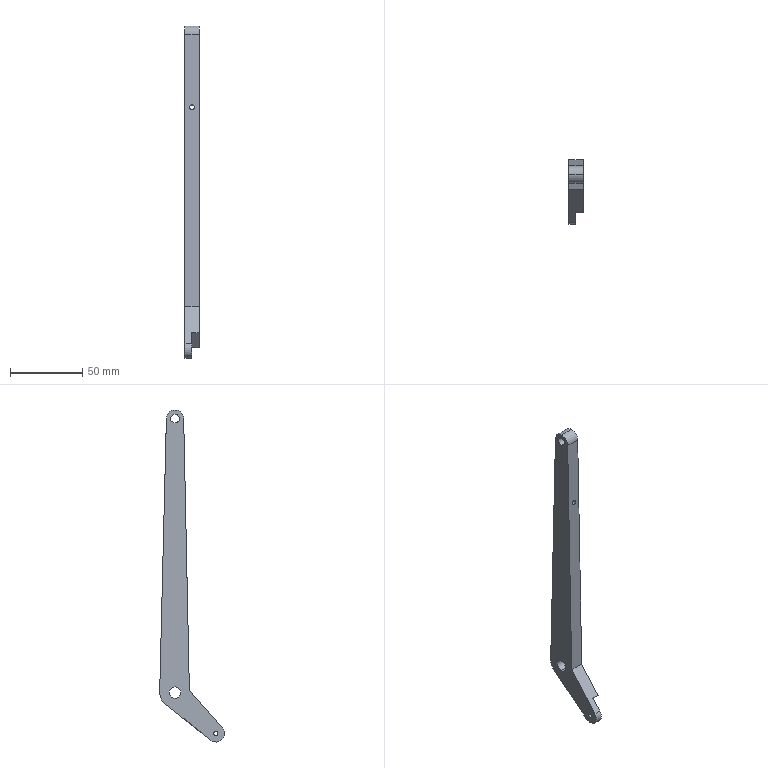Part | STEP file | 11-FG-B05011 | 1 solid | 20 faces | box 9.8 x 44.825 x 230.182 mm | volume 35809 mm3 | cylinder 12 | plane 8 | commonest cylinder face diameters 3 x2 3.3 x2 6 x2 8 x2 12 x2 11.795 x1
STEP:
#1=CARTESIAN_POINT('',(4.9,-7.09,137.958));
#2=VERTEX_POINT('',#1);
#3=CARTESIAN_POINT('',(4.9,-7.021,141.261));
#4=VERTEX_POINT('',#3);
#5=CARTESIAN_POINT('',(4.9,-7.09,137.958));
#6=CARTESIAN_POINT('',(1.6,-7.09,137.958));
#7=CARTESIAN_POINT('',(1.6,-7.021,141.261));
#8=CARTESIAN_POINT('',(4.9,-7.021,141.261));
#9=(BOUNDED_CURVE()B_SPLINE_CURVE(3,(#5,#6,#7,#8),.UNSPECIFIED.,.F.,.F.)B_SPLINE_CURVE_WITH_KNOTS((4,4),(3.142,6.283),.UNSPECIFIED.)CURVE()GEOMETRIC_REPRESENTATION_ITEM()RATIONAL_B_SPLINE_CURVE((1.,0.3333,0.3333,1.))REPRESENTATION_ITEM(''));
#10=EDGE_CURVE('',#2,#4,#9,.T.);
#11=ORIENTED_EDGE('',*,*,#10,.F.);
#12=CARTESIAN_POINT('',(4.9,7.263,138.309));
#13=VERTEX_POINT('',#12);
#14=CARTESIAN_POINT('',(4.9,7.263,138.309));
#15=DIRECTION('',(0.,0.9997,0.02443));
#16=VECTOR('',#15,1000.);
#17=LINE('',#14,#16);
#18=EDGE_CURVE('',#2,#13,#17,.T.);
#19=ORIENTED_EDGE('',*,*,#18,.T.);
#20=CARTESIAN_POINT('',(4.9,7.183,141.608));
#21=VERTEX_POINT('',#20);
#22=CARTESIAN_POINT('',(4.9,7.223,139.958));
#23=DIRECTION('',(0.,0.9997,0.02443));
#24=DIRECTION('',(0.,-0.02443,0.9997));
#25=AXIS2_PLACEMENT_3D('',#22,#23,#24);
#26=CIRCLE('',#25,1.65);
#27=EDGE_CURVE('',#13,#21,#26,.T.);
#28=ORIENTED_EDGE('',*,*,#27,.T.);
#29=CARTESIAN_POINT('',(4.9,7.183,141.608));
#30=DIRECTION('',(0.,0.9997,0.02443));
#31=VECTOR('',#30,1000.);
#32=LINE('',#29,#31);
#33=EDGE_CURVE('',#4,#21,#32,.T.);
#34=ORIENTED_EDGE('',*,*,#33,.F.);
#35=EDGE_LOOP('',(#11,#19,#28,#34));
#36=FACE_OUTER_BOUND('',#35,.T.);
#37=CARTESIAN_POINT('',(4.9,7.223,139.958));
#38=DIRECTION('',(0.,0.9997,0.02443));
#39=DIRECTION('',(0.,-0.02443,0.9997));
#40=AXIS2_PLACEMENT_3D('',#37,#38,#39);
#41=CYLINDRICAL_SURFACE('',#40,1.65);
#42=ADVANCED_FACE('',(#36),#41,.F.);
#43=CARTESIAN_POINT('',(9.8,0.,193.));
#44=VERTEX_POINT('',#43);
#45=CARTESIAN_POINT('',(9.8,0.,187.));
#46=VERTEX_POINT('',#45);
#47=CARTESIAN_POINT('',(9.8,0.,190.));
#48=DIRECTION('',(1.,0.,0.));
#49=DIRECTION('',(0.,0.,-1.));
#50=AXIS2_PLACEMENT_3D('',#47,#48,#49);
#51=CIRCLE('',#50,3.);
#52=EDGE_CURVE('',#44,#46,#51,.T.);
#53=ORIENTED_EDGE('',*,*,#52,.T.);
#54=CARTESIAN_POINT('',(0.,0.,187.));
#55=VERTEX_POINT('',#54);
#56=CARTESIAN_POINT('',(9.8,0.,187.));
#57=DIRECTION('',(-1.,0.,0.));
#58=VECTOR('',#57,1000.);
#59=LINE('',#56,#58);
#60=EDGE_CURVE('',#46,#55,#59,.T.);
#61=ORIENTED_EDGE('',*,*,#60,.T.);
#62=CARTESIAN_POINT('',(0.,0.,193.));
#63=VERTEX_POINT('',#62);
#64=CARTESIAN_POINT('',(0.,0.,190.));
#65=DIRECTION('',(1.,0.,0.));
#66=DIRECTION('',(0.,0.,-1.));
#67=AXIS2_PLACEMENT_3D('',#64,#65,#66);
#68=CIRCLE('',#67,3.);
#69=EDGE_CURVE('',#63,#55,#68,.T.);
#70=ORIENTED_EDGE('',*,*,#69,.F.);
#71=CARTESIAN_POINT('',(9.8,0.,193.));
#72=DIRECTION('',(-1.,0.,0.));
#73=VECTOR('',#72,1000.);
#74=LINE('',#71,#73);
#75=EDGE_CURVE('',#44,#63,#74,.T.);
#76=ORIENTED_EDGE('',*,*,#75,.F.);
#77=EDGE_LOOP('',(#53,#61,#70,#76));
#78=FACE_OUTER_BOUND('',#77,.T.);
#79=CARTESIAN_POINT('',(9.8,0.,190.));
#80=DIRECTION('',(-1.,0.,0.));
#81=DIRECTION('',(0.,0.,1.));
#82=AXIS2_PLACEMENT_3D('',#79,#80,#81);
#83=CYLINDRICAL_SURFACE('',#82,3.);
#84=ADVANCED_FACE('',(#78),#83,.F.);
#85=CARTESIAN_POINT('',(9.8,0.,4.));
#86=VERTEX_POINT('',#85);
#87=CARTESIAN_POINT('',(9.8,0.,-4.));
#88=VERTEX_POINT('',#87);
#89=CARTESIAN_POINT('',(9.8,0.,0.));
#90=DIRECTION('',(1.,0.,0.));
#91=DIRECTION('',(0.,0.,-1.));
#92=AXIS2_PLACEMENT_3D('',#89,#90,#91);
#93=CIRCLE('',#92,4.);
#94=EDGE_CURVE('',#86,#88,#93,.T.);
#95=ORIENTED_EDGE('',*,*,#94,.T.);
#96=CARTESIAN_POINT('',(0.,0.,-4.));
#97=VERTEX_POINT('',#96);
#98=CARTESIAN_POINT('',(9.8,0.,-4.));
#99=DIRECTION('',(-1.,0.,0.));
#100=VECTOR('',#99,1000.);
#101=LINE('',#98,#100);
#102=EDGE_CURVE('',#88,#97,#101,.T.);
#103=ORIENTED_EDGE('',*,*,#102,.T.);
#104=CARTESIAN_POINT('',(0.,0.,4.));
#105=VERTEX_POINT('',#104);
#106=CARTESIAN_POINT('',(0.,0.,0.));
#107=DIRECTION('',(1.,0.,0.));
#108=DIRECTION('',(0.,0.,-1.));
#109=AXIS2_PLACEMENT_3D('',#106,#107,#108);
#110=CIRCLE('',#109,4.);
#111=EDGE_CURVE('',#105,#97,#110,.T.);
#112=ORIENTED_EDGE('',*,*,#111,.F.);
#113=CARTESIAN_POINT('',(9.8,0.,4.));
#114=DIRECTION('',(-1.,0.,0.));
#115=VECTOR('',#114,1000.);
#116=LINE('',#113,#115);
#117=EDGE_CURVE('',#86,#105,#116,.T.);
#118=ORIENTED_EDGE('',*,*,#117,.F.);
#119=EDGE_LOOP('',(#95,#103,#112,#118));
#120=FACE_OUTER_BOUND('',#119,.T.);
#121=CARTESIAN_POINT('',(9.8,0.,0.));
#122=DIRECTION('',(-1.,0.,0.));
#123=DIRECTION('',(0.,0.,1.));
#124=AXIS2_PLACEMENT_3D('',#121,#122,#123);
#125=CYLINDRICAL_SURFACE('',#124,4.);
#126=ADVANCED_FACE('',(#120),#125,.F.);
#127=CARTESIAN_POINT('',(9.8,0.,196.));
#128=VERTEX_POINT('',#127);
#129=CARTESIAN_POINT('',(9.8,-6.,190.));
#130=VERTEX_POINT('',#129);
#131=CARTESIAN_POINT('',(9.8,0.,190.));
#132=DIRECTION('',(1.,0.,0.));
#133=DIRECTION('',(0.,0.,-1.));
#134=AXIS2_PLACEMENT_3D('',#131,#132,#133);
#135=CIRCLE('',#134,6.);
#136=EDGE_CURVE('',#128,#130,#135,.T.);
#137=ORIENTED_EDGE('',*,*,#136,.F.);
#138=CARTESIAN_POINT('',(0.,0.,196.));
#139=VERTEX_POINT('',#138);
#140=CARTESIAN_POINT('',(9.8,0.,196.));
#141=DIRECTION('',(-1.,0.,0.));
#142=VECTOR('',#141,1000.);
#143=LINE('',#140,#142);
#144=EDGE_CURVE('',#128,#139,#143,.T.);
#145=ORIENTED_EDGE('',*,*,#144,.T.);
#146=CARTESIAN_POINT('',(0.,-6.,190.));
#147=VERTEX_POINT('',#146);
#148=CARTESIAN_POINT('',(0.,0.,190.));
#149=DIRECTION('',(1.,0.,0.));
#150=DIRECTION('',(0.,0.,-1.));
#151=AXIS2_PLACEMENT_3D('',#148,#149,#150);
#152=CIRCLE('',#151,6.);
#153=EDGE_CURVE('',#139,#147,#152,.T.);
#154=ORIENTED_EDGE('',*,*,#153,.T.);
#155=CARTESIAN_POINT('',(9.8,-6.,190.));
#156=DIRECTION('',(-1.,0.,0.));
#157=VECTOR('',#156,1000.);
#158=LINE('',#155,#157);
#159=EDGE_CURVE('',#130,#147,#158,.T.);
#160=ORIENTED_EDGE('',*,*,#159,.F.);
#161=EDGE_LOOP('',(#137,#145,#154,#160));
#162=FACE_OUTER_BOUND('',#161,.T.);
#163=CARTESIAN_POINT('',(9.8,0.,190.));
#164=DIRECTION('',(-1.,0.,0.));
#165=DIRECTION('',(0.,0.,1.));
#166=AXIS2_PLACEMENT_3D('',#163,#164,#165);
#167=CYLINDRICAL_SURFACE('',#166,6.);
#168=ADVANCED_FACE('',(#162),#167,.T.);
#169=CARTESIAN_POINT('',(4.8,-28.284,-26.784));
#170=VERTEX_POINT('',#169);
#171=CARTESIAN_POINT('',(4.8,-28.284,-29.784));
#172=VERTEX_POINT('',#171);
#173=CARTESIAN_POINT('',(4.8,-28.284,-28.284));
#174=DIRECTION('',(1.,0.,0.));
#175=DIRECTION('',(0.,0.,-1.));
#176=AXIS2_PLACEMENT_3D('',#173,#174,#175);
#177=CIRCLE('',#176,1.5);
#178=EDGE_CURVE('',#170,#172,#177,.T.);
#179=ORIENTED_EDGE('',*,*,#178,.T.);
#180=CARTESIAN_POINT('',(0.,-28.284,-29.784));
#181=VERTEX_POINT('',#180);
#182=CARTESIAN_POINT('',(9.8,-28.284,-29.784));
#183=DIRECTION('',(-1.,0.,0.));
#184=VECTOR('',#183,1000.);
#185=LINE('',#182,#184);
#186=EDGE_CURVE('',#172,#181,#185,.T.);
#187=ORIENTED_EDGE('',*,*,#186,.T.);
#188=CARTESIAN_POINT('',(0.,-28.284,-26.784));
#189=VERTEX_POINT('',#188);
#190=CARTESIAN_POINT('',(0.,-28.284,-28.284));
#191=DIRECTION('',(1.,0.,0.));
#192=DIRECTION('',(0.,0.,-1.));
#193=AXIS2_PLACEMENT_3D('',#190,#191,#192);
#194=CIRCLE('',#193,1.5);
#195=EDGE_CURVE('',#189,#181,#194,.T.);
#196=ORIENTED_EDGE('',*,*,#195,.F.);
#197=CARTESIAN_POINT('',(9.8,-28.284,-26.784));
#198=DIRECTION('',(-1.,0.,0.));
#199=VECTOR('',#198,1000.);
#200=LINE('',#197,#199);
#201=EDGE_CURVE('',#170,#189,#200,.T.);
#202=ORIENTED_EDGE('',*,*,#201,.F.);
#203=EDGE_LOOP('',(#179,#187,#196,#202));
#204=FACE_OUTER_BOUND('',#203,.T.);
#205=CARTESIAN_POINT('',(9.8,-28.284,-28.284));
#206=DIRECTION('',(-1.,0.,0.));
#207=DIRECTION('',(0.,0.,1.));
#208=AXIS2_PLACEMENT_3D('',#205,#206,#207);
#209=CYLINDRICAL_SURFACE('',#208,1.5);
#210=ADVANCED_FACE('',(#204),#209,.F.);
#211=CARTESIAN_POINT('',(4.8,-32.722,-24.4));
#212=VERTEX_POINT('',#211);
#213=CARTESIAN_POINT('',(4.8,-24.595,-32.885));
#214=VERTEX_POINT('',#213);
#215=CARTESIAN_POINT('',(4.8,-28.284,-28.284));
#216=DIRECTION('',(1.,0.,0.));
#217=DIRECTION('',(0.,0.,-1.));
#218=AXIS2_PLACEMENT_3D('',#215,#216,#217);
#219=CIRCLE('',#218,5.897);
#220=EDGE_CURVE('',#212,#214,#219,.T.);
#221=ORIENTED_EDGE('',*,*,#220,.F.);
#222=CARTESIAN_POINT('',(0.,-32.722,-24.4));
#223=VERTEX_POINT('',#222);
#224=CARTESIAN_POINT('',(9.8,-32.722,-24.4));
#225=DIRECTION('',(-1.,0.,0.));
#226=VECTOR('',#225,1000.);
#227=LINE('',#224,#226);
#228=EDGE_CURVE('',#212,#223,#227,.T.);
#229=ORIENTED_EDGE('',*,*,#228,.T.);
#230=CARTESIAN_POINT('',(0.,-24.595,-32.885));
#231=VERTEX_POINT('',#230);
#232=CARTESIAN_POINT('',(0.,-28.284,-28.284));
#233=DIRECTION('',(1.,0.,0.));
#234=DIRECTION('',(0.,0.,-1.));
#235=AXIS2_PLACEMENT_3D('',#232,#233,#234);
#236=CIRCLE('',#235,5.897);
#237=EDGE_CURVE('',#223,#231,#236,.T.);
#238=ORIENTED_EDGE('',*,*,#237,.T.);
#239=CARTESIAN_POINT('',(9.8,-24.595,-32.885));
#240=DIRECTION('',(-1.,0.,0.));
#241=VECTOR('',#240,1000.);
#242=LINE('',#239,#241);
#243=EDGE_CURVE('',#214,#231,#242,.T.);
#244=ORIENTED_EDGE('',*,*,#243,.F.);
#245=EDGE_LOOP('',(#221,#229,#238,#244));
#246=FACE_OUTER_BOUND('',#245,.T.);
#247=CARTESIAN_POINT('',(9.8,-28.284,-28.284));
#248=DIRECTION('',(-1.,0.,0.));
#249=DIRECTION('',(0.,0.,1.));
#250=AXIS2_PLACEMENT_3D('',#247,#248,#249);
#251=CYLINDRICAL_SURFACE('',#250,5.897);
#252=ADVANCED_FACE('',(#246),#251,.T.);
#253=ORIENTED_EDGE('',*,*,#186,.F.);
#254=CARTESIAN_POINT('',(4.8,-28.284,-28.284));
#255=DIRECTION('',(1.,0.,0.));
#256=DIRECTION('',(0.,0.,-1.));
#257=AXIS2_PLACEMENT_3D('',#254,#255,#256);
#258=CIRCLE('',#257,1.5);
#259=EDGE_CURVE('',#172,#170,#258,.T.);
#260=ORIENTED_EDGE('',*,*,#259,.T.);
#261=ORIENTED_EDGE('',*,*,#201,.T.);
#262=CARTESIAN_POINT('',(0.,-28.284,-28.284));
#263=DIRECTION('',(1.,0.,0.));
#264=DIRECTION('',(0.,0.,-1.));
#265=AXIS2_PLACEMENT_3D('',#262,#263,#264);
#266=CIRCLE('',#265,1.5);
#267=EDGE_CURVE('',#181,#189,#266,.T.);
#268=ORIENTED_EDGE('',*,*,#267,.F.);
#269=EDGE_LOOP('',(#253,#260,#261,#268));
#270=FACE_OUTER_BOUND('',#269,.T.);
#271=CARTESIAN_POINT('',(9.8,-28.284,-28.284));
#272=DIRECTION('',(-1.,0.,0.));
#273=DIRECTION('',(0.,0.,1.));
#274=AXIS2_PLACEMENT_3D('',#271,#272,#273);
#275=CYLINDRICAL_SURFACE('',#274,1.5);
#276=ADVANCED_FACE('',(#270),#275,.F.);
#277=CARTESIAN_POINT('',(9.8,-17.236,-26.984));
#278=VERTEX_POINT('',#277);
#279=CARTESIAN_POINT('',(9.8,-26.006,-16.728));
#280=VERTEX_POINT('',#279);
#281=CARTESIAN_POINT('',(9.8,-17.236,-26.984));
#282=DIRECTION('',(0.,-0.6499,0.76));
#283=VECTOR('',#282,1000.);
#284=LINE('',#281,#283);
#285=EDGE_CURVE('',#278,#280,#284,.T.);
#286=ORIENTED_EDGE('',*,*,#285,.F.);
#287=CARTESIAN_POINT('',(9.8,8.61,-6.257));
#288=VERTEX_POINT('',#287);
#289=CARTESIAN_POINT('',(9.8,8.61,-6.257));
#290=DIRECTION('',(0.,0.7801,0.6256));
#291=VECTOR('',#290,1000.);
#292=LINE('',#289,#291);
#293=EDGE_CURVE('',#278,#288,#292,.T.);
#294=ORIENTED_EDGE('',*,*,#293,.T.);
#295=CARTESIAN_POINT('',(9.8,10.643,0.));
#296=VERTEX_POINT('',#295);
#297=CARTESIAN_POINT('',(9.8,0.,0.));
#298=DIRECTION('',(1.,0.,0.));
#299=DIRECTION('',(0.,0.,-1.));
#300=AXIS2_PLACEMENT_3D('',#297,#298,#299);
#301=CIRCLE('',#300,10.643);
#302=EDGE_CURVE('',#288,#296,#301,.T.);
#303=ORIENTED_EDGE('',*,*,#302,.T.);
#304=CARTESIAN_POINT('',(9.8,6.,190.));
#305=VERTEX_POINT('',#304);
#306=CARTESIAN_POINT('',(9.8,10.643,0.));
#307=DIRECTION('',(0.,-0.02443,0.9997));
#308=VECTOR('',#307,1000.);
#309=LINE('',#306,#308);
#310=EDGE_CURVE('',#296,#305,#309,.T.);
#311=ORIENTED_EDGE('',*,*,#310,.T.);
#312=CARTESIAN_POINT('',(9.8,0.,190.));
#313=DIRECTION('',(1.,0.,0.));
#314=DIRECTION('',(0.,0.,-1.));
#315=AXIS2_PLACEMENT_3D('',#312,#313,#314);
#316=CIRCLE('',#315,6.);
#317=EDGE_CURVE('',#305,#128,#316,.T.);
#318=ORIENTED_EDGE('',*,*,#317,.T.);
#319=ORIENTED_EDGE('',*,*,#136,.T.);
#320=CARTESIAN_POINT('',(9.8,-9.946,1.617));
#321=VERTEX_POINT('',#320);
#322=CARTESIAN_POINT('',(9.8,-9.946,1.617));
#323=DIRECTION('',(0.,-0.02094,-0.9998));
#324=VECTOR('',#323,1000.);
#325=LINE('',#322,#324);
#326=EDGE_CURVE('',#130,#321,#325,.T.);
#327=ORIENTED_EDGE('',*,*,#326,.T.);
#328=CARTESIAN_POINT('',(9.8,-9.946,1.617));
#329=DIRECTION('',(0.,-0.6587,-0.7524));
#330=VECTOR('',#329,1000.);
#331=LINE('',#328,#330);
#332=EDGE_CURVE('',#321,#280,#331,.T.);
#333=ORIENTED_EDGE('',*,*,#332,.T.);
#334=EDGE_LOOP('',(#286,#294,#303,#311,#318,#319,#327,#333));
#335=FACE_OUTER_BOUND('',#334,.T.);
#336=ORIENTED_EDGE('',*,*,#52,.F.);
#337=CARTESIAN_POINT('',(9.8,0.,190.));
#338=DIRECTION('',(1.,0.,0.));
#339=DIRECTION('',(0.,0.,-1.));
#340=AXIS2_PLACEMENT_3D('',#337,#338,#339);
#341=CIRCLE('',#340,3.);
#342=EDGE_CURVE('',#46,#44,#341,.T.);
#343=ORIENTED_EDGE('',*,*,#342,.F.);
#344=EDGE_LOOP('',(#336,#343));
#345=FACE_BOUND('',#344,.T.);
#346=ORIENTED_EDGE('',*,*,#94,.F.);
#347=CARTESIAN_POINT('',(9.8,0.,0.));
#348=DIRECTION('',(1.,0.,0.));
#349=DIRECTION('',(0.,0.,-1.));
#350=AXIS2_PLACEMENT_3D('',#347,#348,#349);
#351=CIRCLE('',#350,4.);
#352=EDGE_CURVE('',#88,#86,#351,.T.);
#353=ORIENTED_EDGE('',*,*,#352,.F.);
#354=EDGE_LOOP('',(#346,#353));
#355=FACE_BOUND('',#354,.T.);
#356=CARTESIAN_POINT('',(9.8,0.,0.));
#357=DIRECTION('',(1.,0.,0.));
#358=DIRECTION('',(0.,0.,-1.));
#359=AXIS2_PLACEMENT_3D('',#356,#357,#358);
#360=PLANE('',#359);
#361=ADVANCED_FACE('',(#335,#345,#355),#360,.T.);
#362=CARTESIAN_POINT('',(0.,8.61,-6.257));
#363=VERTEX_POINT('',#362);
#364=CARTESIAN_POINT('',(0.,10.643,0.));
#365=VERTEX_POINT('',#364);
#366=CARTESIAN_POINT('',(0.,0.,0.));
#367=DIRECTION('',(1.,0.,0.));
#368=DIRECTION('',(0.,0.,-1.));
#369=AXIS2_PLACEMENT_3D('',#366,#367,#368);
#370=CIRCLE('',#369,10.643);
#371=EDGE_CURVE('',#363,#365,#370,.T.);
#372=ORIENTED_EDGE('',*,*,#371,.F.);
#373=CARTESIAN_POINT('',(0.,8.61,-6.257));
#374=DIRECTION('',(0.,0.7801,0.6256));
#375=VECTOR('',#374,1000.);
#376=LINE('',#373,#375);
#377=EDGE_CURVE('',#231,#363,#376,.T.);
#378=ORIENTED_EDGE('',*,*,#377,.F.);
#379=ORIENTED_EDGE('',*,*,#237,.F.);
#380=CARTESIAN_POINT('',(0.,-9.946,1.617));
#381=VERTEX_POINT('',#380);
#382=CARTESIAN_POINT('',(0.,-9.946,1.617));
#383=DIRECTION('',(0.,-0.6587,-0.7524));
#384=VECTOR('',#383,1000.);
#385=LINE('',#382,#384);
#386=EDGE_CURVE('',#381,#223,#385,.T.);
#387=ORIENTED_EDGE('',*,*,#386,.F.);
#388=CARTESIAN_POINT('',(0.,-9.946,1.617));
#389=DIRECTION('',(0.,-0.02094,-0.9998));
#390=VECTOR('',#389,1000.);
#391=LINE('',#388,#390);
#392=EDGE_CURVE('',#147,#381,#391,.T.);
#393=ORIENTED_EDGE('',*,*,#392,.F.);
#394=ORIENTED_EDGE('',*,*,#153,.F.);
#395=CARTESIAN_POINT('',(0.,6.,190.));
#396=VERTEX_POINT('',#395);
#397=CARTESIAN_POINT('',(0.,0.,190.));
#398=DIRECTION('',(1.,0.,0.));
#399=DIRECTION('',(0.,0.,-1.));
#400=AXIS2_PLACEMENT_3D('',#397,#398,#399);
#401=CIRCLE('',#400,6.);
#402=EDGE_CURVE('',#396,#139,#401,.T.);
#403=ORIENTED_EDGE('',*,*,#402,.F.);
#404=CARTESIAN_POINT('',(0.,10.643,0.));
#405=DIRECTION('',(0.,-0.02443,0.9997));
#406=VECTOR('',#405,1000.);
#407=LINE('',#404,#406);
#408=EDGE_CURVE('',#365,#396,#407,.T.);
#409=ORIENTED_EDGE('',*,*,#408,.F.);
#410=EDGE_LOOP('',(#372,#378,#379,#387,#393,#394,#403,#409));
#411=FACE_OUTER_BOUND('',#410,.T.);
#412=ORIENTED_EDGE('',*,*,#111,.T.);
#413=CARTESIAN_POINT('',(0.,0.,0.));
#414=DIRECTION('',(1.,0.,0.));
#415=DIRECTION('',(0.,0.,-1.));
#416=AXIS2_PLACEMENT_3D('',#413,#414,#415);
#417=CIRCLE('',#416,4.);
#418=EDGE_CURVE('',#97,#105,#417,.T.);
#419=ORIENTED_EDGE('',*,*,#418,.T.);
#420=EDGE_LOOP('',(#412,#419));
#421=FACE_BOUND('',#420,.T.);
#422=ORIENTED_EDGE('',*,*,#69,.T.);
#423=CARTESIAN_POINT('',(0.,0.,190.));
#424=DIRECTION('',(1.,0.,0.));
#425=DIRECTION('',(0.,0.,-1.));
#426=AXIS2_PLACEMENT_3D('',#423,#424,#425);
#427=CIRCLE('',#426,3.);
#428=EDGE_CURVE('',#55,#63,#427,.T.);
#429=ORIENTED_EDGE('',*,*,#428,.T.);
#430=EDGE_LOOP('',(#422,#429));
#431=FACE_BOUND('',#430,.T.);
#432=ORIENTED_EDGE('',*,*,#195,.T.);
#433=ORIENTED_EDGE('',*,*,#267,.T.);
#434=EDGE_LOOP('',(#432,#433));
#435=FACE_BOUND('',#434,.T.);
#436=CARTESIAN_POINT('',(0.,0.,0.));
#437=DIRECTION('',(1.,0.,0.));
#438=DIRECTION('',(0.,0.,-1.));
#439=AXIS2_PLACEMENT_3D('',#436,#437,#438);
#440=PLANE('',#439);
#441=ADVANCED_FACE('',(#411,#421,#431,#435),#440,.F.);
#442=ORIENTED_EDGE('',*,*,#371,.T.);
#443=CARTESIAN_POINT('',(9.8,10.643,0.));
#444=DIRECTION('',(-1.,0.,0.));
#445=VECTOR('',#444,1000.);
#446=LINE('',#443,#445);
#447=EDGE_CURVE('',#296,#365,#446,.T.);
#448=ORIENTED_EDGE('',*,*,#447,.F.);
#449=ORIENTED_EDGE('',*,*,#302,.F.);
#450=CARTESIAN_POINT('',(9.8,8.61,-6.257));
#451=DIRECTION('',(-1.,0.,0.));
#452=VECTOR('',#451,1000.);
#453=LINE('',#450,#452);
#454=EDGE_CURVE('',#288,#363,#453,.T.);
#455=ORIENTED_EDGE('',*,*,#454,.T.);
#456=EDGE_LOOP('',(#442,#448,#449,#455));
#457=FACE_OUTER_BOUND('',#456,.T.);
#458=CARTESIAN_POINT('',(9.8,0.,0.));
#459=DIRECTION('',(-1.,0.,0.));
#460=DIRECTION('',(0.,0.,1.));
#461=AXIS2_PLACEMENT_3D('',#458,#459,#460);
#462=CYLINDRICAL_SURFACE('',#461,10.643);
#463=ADVANCED_FACE('',(#457),#462,.T.);
#464=CARTESIAN_POINT('',(4.9,7.223,139.958));
#465=DIRECTION('',(0.,0.9997,0.02443));
#466=DIRECTION('',(0.,-0.02443,0.9997));
#467=AXIS2_PLACEMENT_3D('',#464,#465,#466);
#468=CIRCLE('',#467,1.65);
#469=EDGE_CURVE('',#21,#13,#468,.T.);
#470=ORIENTED_EDGE('',*,*,#469,.F.);
#471=ORIENTED_EDGE('',*,*,#27,.F.);
#472=EDGE_LOOP('',(#470,#471));
#473=FACE_BOUND('',#472,.T.);
#474=ORIENTED_EDGE('',*,*,#408,.T.);
#475=CARTESIAN_POINT('',(9.8,6.,190.));
#476=DIRECTION('',(-1.,0.,0.));
#477=VECTOR('',#476,1000.);
#478=LINE('',#475,#477);
#479=EDGE_CURVE('',#305,#396,#478,.T.);
#480=ORIENTED_EDGE('',*,*,#479,.F.);
#481=ORIENTED_EDGE('',*,*,#310,.F.);
#482=ORIENTED_EDGE('',*,*,#447,.T.);
#483=EDGE_LOOP('',(#474,#480,#481,#482));
#484=FACE_OUTER_BOUND('',#483,.T.);
#485=CARTESIAN_POINT('',(9.8,10.643,0.));
#486=DIRECTION('',(0.,-0.9997,-0.02443));
#487=DIRECTION('',(0.,0.02443,-0.9997));
#488=AXIS2_PLACEMENT_3D('',#485,#486,#487);
#489=PLANE('',#488);
#490=ADVANCED_FACE('',(#473,#484),#489,.F.);
#491=ORIENTED_EDGE('',*,*,#144,.F.);
#492=ORIENTED_EDGE('',*,*,#317,.F.);
#493=ORIENTED_EDGE('',*,*,#479,.T.);
#494=ORIENTED_EDGE('',*,*,#402,.T.);
#495=EDGE_LOOP('',(#491,#492,#493,#494));
#496=FACE_OUTER_BOUND('',#495,.T.);
#497=CARTESIAN_POINT('',(9.8,0.,190.));
#498=DIRECTION('',(-1.,0.,0.));
#499=DIRECTION('',(0.,0.,1.));
#500=AXIS2_PLACEMENT_3D('',#497,#498,#499);
#501=CYLINDRICAL_SURFACE('',#500,6.);
#502=ADVANCED_FACE('',(#496),#501,.T.);
#503=CARTESIAN_POINT('',(4.9,-7.021,141.261));
#504=CARTESIAN_POINT('',(8.2,-7.021,141.261));
#505=CARTESIAN_POINT('',(8.2,-7.09,137.958));
#506=CARTESIAN_POINT('',(4.9,-7.09,137.958));
#507=(BOUNDED_CURVE()B_SPLINE_CURVE(3,(#503,#504,#505,#506),.UNSPECIFIED.,.F.,.F.)B_SPLINE_CURVE_WITH_KNOTS((4,4),(0.,3.142),.UNSPECIFIED.)CURVE()GEOMETRIC_REPRESENTATION_ITEM()RATIONAL_B_SPLINE_CURVE((1.,0.3333,0.3333,1.))REPRESENTATION_ITEM(''));
#508=EDGE_CURVE('',#4,#2,#507,.T.);
#509=ORIENTED_EDGE('',*,*,#508,.T.);
#510=ORIENTED_EDGE('',*,*,#10,.T.);
#511=EDGE_LOOP('',(#509,#510));
#512=FACE_BOUND('',#511,.T.);
#513=ORIENTED_EDGE('',*,*,#392,.T.);
#514=CARTESIAN_POINT('',(9.8,-9.946,1.617));
#515=DIRECTION('',(-1.,0.,0.));
#516=VECTOR('',#515,1000.);
#517=LINE('',#514,#516);
#518=EDGE_CURVE('',#321,#381,#517,.T.);
#519=ORIENTED_EDGE('',*,*,#518,.F.);
#520=ORIENTED_EDGE('',*,*,#326,.F.);
#521=ORIENTED_EDGE('',*,*,#159,.T.);
#522=EDGE_LOOP('',(#513,#519,#520,#521));
#523=FACE_OUTER_BOUND('',#522,.T.);
#524=CARTESIAN_POINT('',(9.8,-9.946,1.617));
#525=DIRECTION('',(0.,0.9998,-0.02094));
#526=DIRECTION('',(0.,0.02094,0.9998));
#527=AXIS2_PLACEMENT_3D('',#524,#525,#526);
#528=PLANE('',#527);
#529=ADVANCED_FACE('',(#512,#523),#528,.F.);
#530=CARTESIAN_POINT('',(4.8,-26.006,-16.728));
#531=VERTEX_POINT('',#530);
#532=CARTESIAN_POINT('',(4.8,-26.006,-16.728));
#533=DIRECTION('',(0.,-0.6587,-0.7524));
#534=VECTOR('',#533,1000.);
#535=LINE('',#532,#534);
#536=EDGE_CURVE('',#531,#212,#535,.T.);
#537=ORIENTED_EDGE('',*,*,#536,.F.);
#538=CARTESIAN_POINT('',(4.8,-26.006,-16.728));
#539=DIRECTION('',(1.,0.,0.));
#540=VECTOR('',#539,1000.);
#541=LINE('',#538,#540);
#542=EDGE_CURVE('',#531,#280,#541,.T.);
#543=ORIENTED_EDGE('',*,*,#542,.T.);
#544=ORIENTED_EDGE('',*,*,#332,.F.);
#545=ORIENTED_EDGE('',*,*,#518,.T.);
#546=ORIENTED_EDGE('',*,*,#386,.T.);
#547=ORIENTED_EDGE('',*,*,#228,.F.);
#548=EDGE_LOOP('',(#537,#543,#544,#545,#546,#547));
#549=FACE_OUTER_BOUND('',#548,.T.);
#550=CARTESIAN_POINT('',(9.8,-9.946,1.617));
#551=DIRECTION('',(0.,0.7524,-0.6587));
#552=DIRECTION('',(0.,0.6587,0.7524));
#553=AXIS2_PLACEMENT_3D('',#550,#551,#552);
#554=PLANE('',#553);
#555=ADVANCED_FACE('',(#549),#554,.F.);
#556=ORIENTED_EDGE('',*,*,#293,.F.);
#557=CARTESIAN_POINT('',(4.8,-17.236,-26.984));
#558=VERTEX_POINT('',#557);
#559=CARTESIAN_POINT('',(4.8,-17.236,-26.984));
#560=DIRECTION('',(1.,0.,0.));
#561=VECTOR('',#560,1000.);
#562=LINE('',#559,#561);
#563=EDGE_CURVE('',#558,#278,#562,.T.);
#564=ORIENTED_EDGE('',*,*,#563,.F.);
#565=CARTESIAN_POINT('',(4.8,-17.236,-26.984));
#566=DIRECTION('',(0.,0.7801,0.6256));
#567=VECTOR('',#566,1000.);
#568=LINE('',#565,#567);
#569=EDGE_CURVE('',#214,#558,#568,.T.);
#570=ORIENTED_EDGE('',*,*,#569,.F.);
#571=ORIENTED_EDGE('',*,*,#243,.T.);
#572=ORIENTED_EDGE('',*,*,#377,.T.);
#573=ORIENTED_EDGE('',*,*,#454,.F.);
#574=EDGE_LOOP('',(#556,#564,#570,#571,#572,#573));
#575=FACE_OUTER_BOUND('',#574,.T.);
#576=CARTESIAN_POINT('',(9.8,8.61,-6.257));
#577=DIRECTION('',(0.,-0.6256,0.7801));
#578=DIRECTION('',(0.,-0.7801,-0.6256));
#579=AXIS2_PLACEMENT_3D('',#576,#577,#578);
#580=PLANE('',#579);
#581=ADVANCED_FACE('',(#575),#580,.F.);
#582=ORIENTED_EDGE('',*,*,#102,.F.);
#583=ORIENTED_EDGE('',*,*,#352,.T.);
#584=ORIENTED_EDGE('',*,*,#117,.T.);
#585=ORIENTED_EDGE('',*,*,#418,.F.);
#586=EDGE_LOOP('',(#582,#583,#584,#585));
#587=FACE_OUTER_BOUND('',#586,.T.);
#588=CARTESIAN_POINT('',(9.8,0.,0.));
#589=DIRECTION('',(-1.,0.,0.));
#590=DIRECTION('',(0.,0.,1.));
#591=AXIS2_PLACEMENT_3D('',#588,#589,#590);
#592=CYLINDRICAL_SURFACE('',#591,4.);
#593=ADVANCED_FACE('',(#587),#592,.F.);
#594=ORIENTED_EDGE('',*,*,#60,.F.);
#595=ORIENTED_EDGE('',*,*,#342,.T.);
#596=ORIENTED_EDGE('',*,*,#75,.T.);
#597=ORIENTED_EDGE('',*,*,#428,.F.);
#598=EDGE_LOOP('',(#594,#595,#596,#597));
#599=FACE_OUTER_BOUND('',#598,.T.);
#600=CARTESIAN_POINT('',(9.8,0.,190.));
#601=DIRECTION('',(-1.,0.,0.));
#602=DIRECTION('',(0.,0.,1.));
#603=AXIS2_PLACEMENT_3D('',#600,#601,#602);
#604=CYLINDRICAL_SURFACE('',#603,3.);
#605=ADVANCED_FACE('',(#599),#604,.F.);
#606=ORIENTED_EDGE('',*,*,#18,.F.);
#607=ORIENTED_EDGE('',*,*,#508,.F.);
#608=ORIENTED_EDGE('',*,*,#33,.T.);
#609=ORIENTED_EDGE('',*,*,#469,.T.);
#610=EDGE_LOOP('',(#606,#607,#608,#609));
#611=FACE_OUTER_BOUND('',#610,.T.);
#612=CARTESIAN_POINT('',(4.9,7.223,139.958));
#613=DIRECTION('',(0.,0.9997,0.02443));
#614=DIRECTION('',(0.,-0.02443,0.9997));
#615=AXIS2_PLACEMENT_3D('',#612,#613,#614);
#616=CYLINDRICAL_SURFACE('',#615,1.65);
#617=ADVANCED_FACE('',(#611),#616,.F.);
#618=ORIENTED_EDGE('',*,*,#178,.F.);
#619=ORIENTED_EDGE('',*,*,#259,.F.);
#620=EDGE_LOOP('',(#618,#619));
#621=FACE_BOUND('',#620,.T.);
#622=ORIENTED_EDGE('',*,*,#220,.T.);
#623=ORIENTED_EDGE('',*,*,#569,.T.);
#624=CARTESIAN_POINT('',(4.8,-17.236,-26.984));
#625=DIRECTION('',(0.,-0.6499,0.76));
#626=VECTOR('',#625,1000.);
#627=LINE('',#624,#626);
#628=EDGE_CURVE('',#558,#531,#627,.T.);
#629=ORIENTED_EDGE('',*,*,#628,.T.);
#630=ORIENTED_EDGE('',*,*,#536,.T.);
#631=EDGE_LOOP('',(#622,#623,#629,#630));
#632=FACE_OUTER_BOUND('',#631,.T.);
#633=CARTESIAN_POINT('',(4.8,0.,0.));
#634=DIRECTION('',(1.,0.,0.));
#635=DIRECTION('',(0.,0.,-1.));
#636=AXIS2_PLACEMENT_3D('',#633,#634,#635);
#637=PLANE('',#636);
#638=ADVANCED_FACE('',(#621,#632),#637,.T.);
#639=ORIENTED_EDGE('',*,*,#285,.T.);
#640=ORIENTED_EDGE('',*,*,#542,.F.);
#641=ORIENTED_EDGE('',*,*,#628,.F.);
#642=ORIENTED_EDGE('',*,*,#563,.T.);
#643=EDGE_LOOP('',(#639,#640,#641,#642));
#644=FACE_OUTER_BOUND('',#643,.T.);
#645=CARTESIAN_POINT('',(4.8,-17.236,-26.984));
#646=DIRECTION('',(0.,0.76,0.6499));
#647=DIRECTION('',(0.,-0.6499,0.76));
#648=AXIS2_PLACEMENT_3D('',#645,#646,#647);
#649=PLANE('',#648);
#650=ADVANCED_FACE('',(#644),#649,.F.);
#651=CLOSED_SHELL('',(#42,#84,#126,#168,#210,#252,#276,#361,#441,#463,#490,#502,#529,#555,#581,#593,#605,#617,#638,#650));
#652=MANIFOLD_SOLID_BREP('',#651);
#653=CARTESIAN_POINT('',(0.,0.,0.));
#654=DIRECTION('',(0.,0.,1.));
#655=DIRECTION('',(1.,0.,0.));
#656=AXIS2_PLACEMENT_3D('',#653,#654,#655);
#657=(LENGTH_UNIT()NAMED_UNIT(*)SI_UNIT(.MILLI.,.METRE.));
#658=UNCERTAINTY_MEASURE_WITH_UNIT(LENGTH_MEASURE(0.00001),#657,'','');
#659=(NAMED_UNIT(*)PLANE_ANGLE_UNIT()SI_UNIT($,.RADIAN.));
#660=(NAMED_UNIT(*)SI_UNIT($,.STERADIAN.)SOLID_ANGLE_UNIT());
#661=(GEOMETRIC_REPRESENTATION_CONTEXT(3)GLOBAL_UNCERTAINTY_ASSIGNED_CONTEXT((#658))GLOBAL_UNIT_ASSIGNED_CONTEXT((#657,#659,#660))REPRESENTATION_CONTEXT('',''));
#662=ADVANCED_BREP_SHAPE_REPRESENTATION('',(#652,#656),#661);